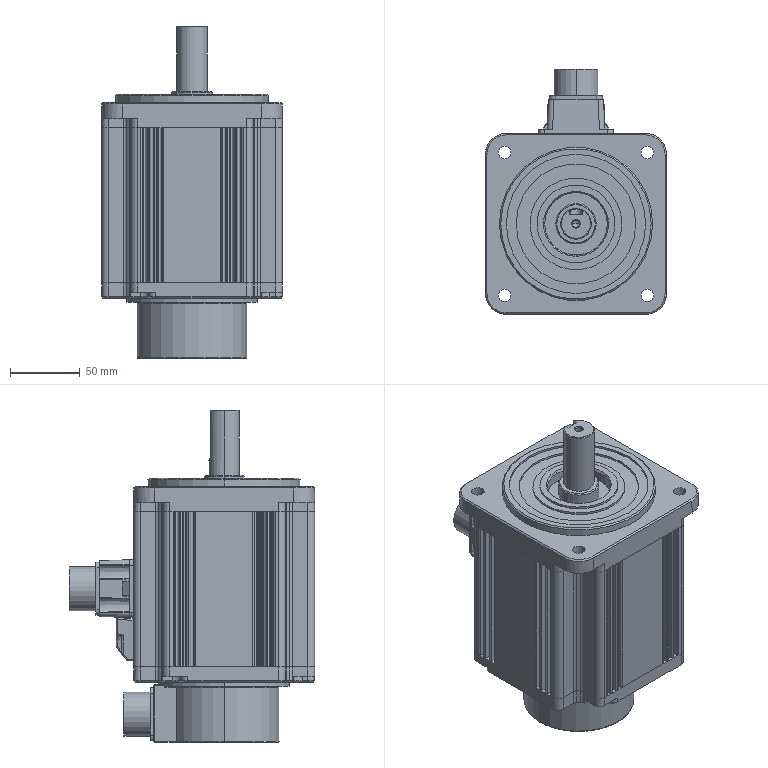Part | SolidWorks | features BaseBody 1 | 1 solid | 614 faces | box 130 x 176.14 x 238.5 mm | volume 2461852 mm3 | plane 282 | cylinder 235 | spline 67 | cone 30 | commonest cylinder face diameters 2 x96 1 x25 9.97 x24 6.017 x18 8 x17 9 x8